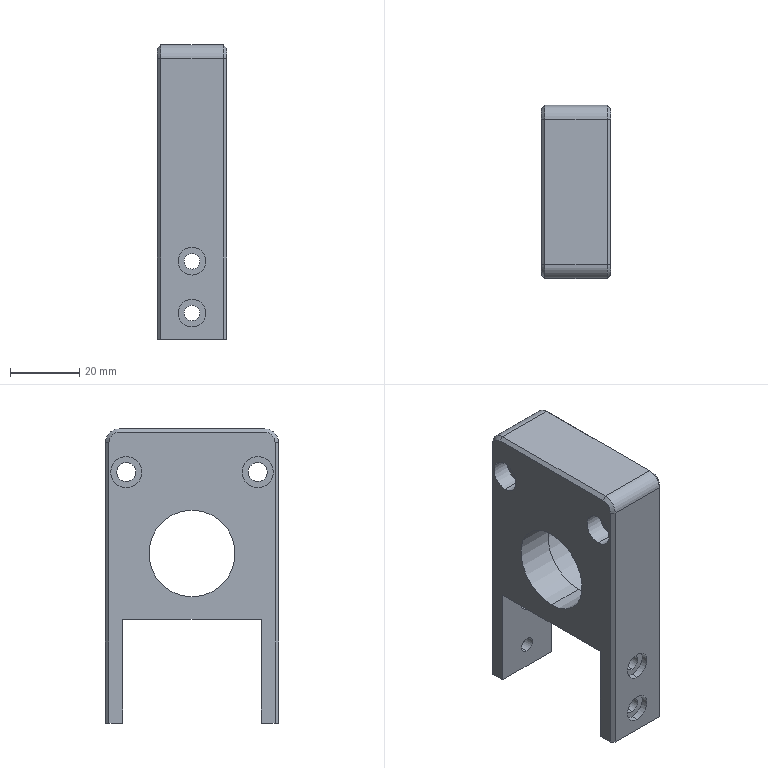Part | STEP file | 1 solid | 57 faces | box 20 x 50 x 85 mm | volume 46036 mm3 | cylinder 30 | plane 23 | cone 4 | commonest cylinder face diameters 8 x10 4.5 x8 5.5 x4 9 x4 25 x2 32 x2